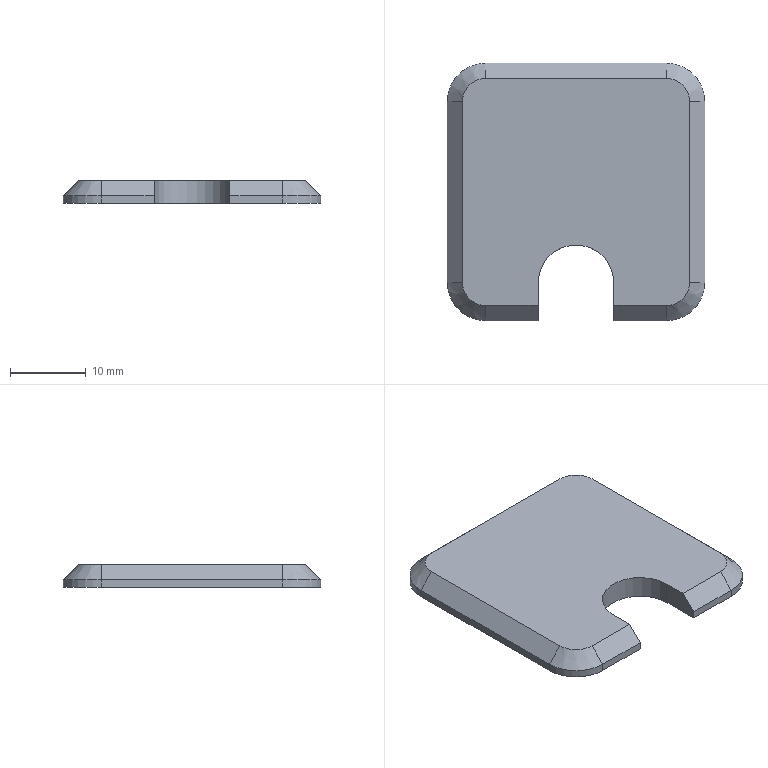Part | STEP file | IN-01-01-01-02 | 1 solid | 23 faces | box 34 x 34 x 3 mm | volume 2909 mm3 | plane 14 | cylinder 5 | cone 4 | commonest cylinder face diameters 10 x5